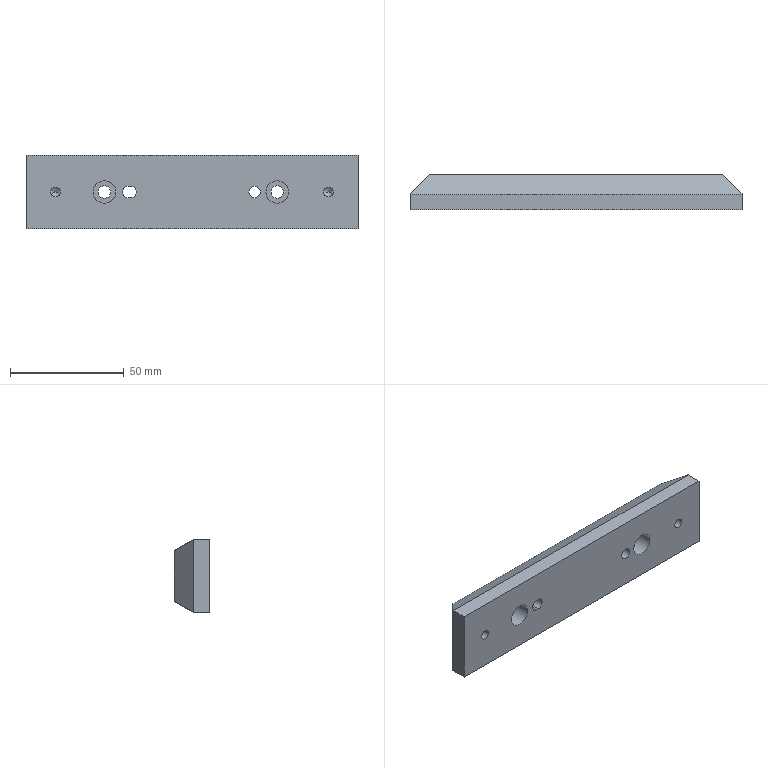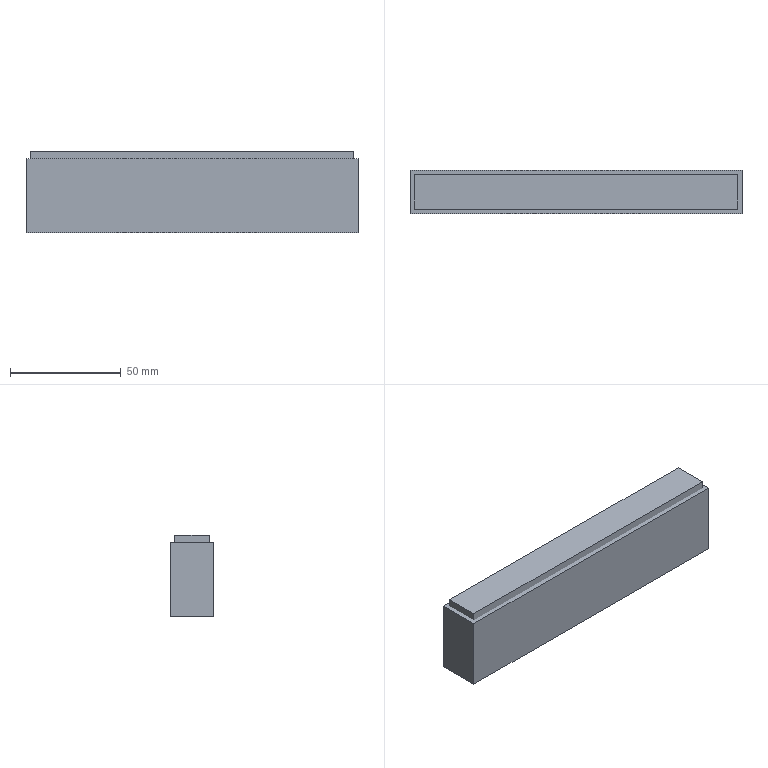CAM job | NX | 3-axis milling, drilling | part box 146 x 15.5 x 32.5 mm | stock box 150 x 19.5 x 37 mm
Tools:
number,name,description,diameter,corner_radius,flute_length,length,flutes
19,D80,Milling Tool-5 Parameters,80.0,0.0,50.0,75.0,2
15,D10,Milling Tool-5 Parameters,10.0,0.0,50.0,75.0,2
1,D6A45,Milling Tool-5 Parameters,6.0,0.0,50.0,75.0,2
14,D10JING,Milling Tool-5 Parameters,10.0,0.0,50.0,75.0,2
4,4.2ZT,Drilling Tool,4.2,0.0,35.0,50.0,2
9,5.5ZT,Drilling Tool,5.5,0.0,35.0,50.0,2
12,D6,Milling Tool-5 Parameters,6.0,0.0,50.0,75.0,2
11,D4,Milling Tool-5 Parameters,4.0,0.0,50.0,75.0,2
16,D6R0.5,Milling Tool-5 Parameters,6.0,0.5,50.0,75.0,2
Operations:
program,operation,operation_type,tool,method,geometry_group,spindle_rpm,surface_speed,feed_per_tooth,feed_cut,feed_plunge,cut_length_mm,path_length_mm,cut_time_min,machine_time_min
1,FLOOR_WALL,VolumeBased25DMillingOperation,D80,METHOD,A,6500.0,1633.0,0.1154,1500.0,100.0,242.0,296.0,0.1613,0.1667
1,ZLEVEL_PROFILE,ZLevelMilling,D10,METHOD,A,9500.0,298.0,0.1579,3000.0,1000.0,6662.248,6734.748,2.252,2.259
1,ZLEVEL_PROFILE_1,ZLevelMilling,D10JING,METHOD,A,9500.0,298.0,0.0789,1500.0,1000.0,396.754,484.754,0.2659,0.2747
1,DRILLING,Operation,D6A45,METHOD,A,9500.0,179.0,0.0132,250.0,0.0,24.0,244.315,0.096,0.118
1,DRILLING_1,Operation,4.2ZT,METHOD,A,2000.0,26.0,0.0625,250.0,0.0,76.247,341.851,0.305,0.3315
1,DRILLING_1_COPY,Operation,5.5ZT,METHOD,A,2000.0,26.0,0.0625,250.0,0.0,42.305,223.669,0.1692,0.1874
1,HOLE_MILLING,CylinderMilling,D6,METHOD,A,9500.0,179.0,0.0789,1500.0,100.0,478.023,693.023,0.3187,0.3402
1,ZLEVEL_PROFILE_COPY,ZLevelMilling,D4,METHOD,A,9500.0,119.0,0.0526,1000.0,1000.0,326.199,579.606,0.3262,0.3515
1,PLANAR_MILL_COPY,PlanarMilling,D6A45,METHOD,A,9500.0,179.0,0.0658,1250.0,100.0,487.024,1031.236,0.3896,0.444
1,刀补,ZLevelMilling,D4,METHOD,A,9500.0,119.0,0.0632,1200.0,1000.0,67.975,327.67,0.057,0.083
2,FLOOR_WALL_COPY,VolumeBased25DMillingOperation,D80,METHOD,B,6500.0,1633.0,0.1154,1500.0,100.0,1190.0,2370.001,0.7933,0.9113
2,ZLEVEL_PROFILE_COPY_1,ZLevelMilling,D6R0.5,METHOD,B,9500.0,298.0,0.1579,3000.0,1000.0,51120.434,51186.934,17.06,17.067
2,PLANAR_MILL_COPY_COPY,PlanarMilling,D6A45,METHOD,B,9500.0,179.0,0.0658,1250.0,100.0,65.732,376.317,0.0526,0.0836